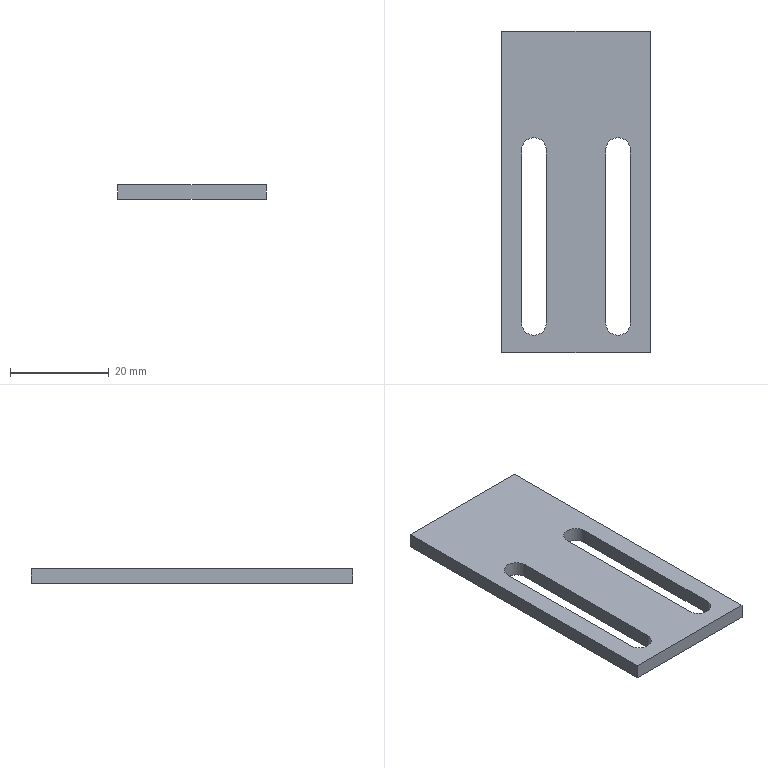Part | SolidWorks | features Extrusion 1, ICE 1, MirrorPattern 1 | 1 solid | 14 faces | box 30 x 65 x 3 mm | volume 4682 mm3 | plane 10 | cylinder 4 | commonest cylinder face diameters 5 x4
STEP:
#1=CARTESIAN_POINT('',(15.,-32.5,3.));
#2=VERTEX_POINT('',#1);
#3=CARTESIAN_POINT('',(15.,32.5,3.));
#4=VERTEX_POINT('',#3);
#5=CARTESIAN_POINT('',(15.,-32.5,3.));
#6=DIRECTION('',(0.,1.,0.));
#7=VECTOR('',#6,1000.);
#8=LINE('',#5,#7);
#9=EDGE_CURVE('',#2,#4,#8,.T.);
#10=ORIENTED_EDGE('',*,*,#9,.T.);
#11=CARTESIAN_POINT('',(-15.,32.5,3.));
#12=VERTEX_POINT('',#11);
#13=CARTESIAN_POINT('',(-15.,32.5,3.));
#14=DIRECTION('',(-1.,0.,0.));
#15=VECTOR('',#14,1000.);
#16=LINE('',#13,#15);
#17=EDGE_CURVE('',#4,#12,#16,.T.);
#18=ORIENTED_EDGE('',*,*,#17,.T.);
#19=CARTESIAN_POINT('',(-15.,-32.5,3.));
#20=VERTEX_POINT('',#19);
#21=CARTESIAN_POINT('',(-15.,-32.5,3.));
#22=DIRECTION('',(0.,-1.,0.));
#23=VECTOR('',#22,1000.);
#24=LINE('',#21,#23);
#25=EDGE_CURVE('',#12,#20,#24,.T.);
#26=ORIENTED_EDGE('',*,*,#25,.T.);
#27=CARTESIAN_POINT('',(-15.,-32.5,3.));
#28=DIRECTION('',(1.,0.,0.));
#29=VECTOR('',#28,1000.);
#30=LINE('',#27,#29);
#31=EDGE_CURVE('',#20,#2,#30,.T.);
#32=ORIENTED_EDGE('',*,*,#31,.T.);
#33=EDGE_LOOP('',(#10,#18,#26,#32));
#34=FACE_OUTER_BOUND('',#33,.T.);
#35=CARTESIAN_POINT('',(-6.,-26.5,3.));
#36=VERTEX_POINT('',#35);
#37=CARTESIAN_POINT('',(-6.,8.5,3.));
#38=VERTEX_POINT('',#37);
#39=CARTESIAN_POINT('',(-6.,-26.5,3.));
#40=DIRECTION('',(0.,1.,0.));
#41=VECTOR('',#40,1000.);
#42=LINE('',#39,#41);
#43=EDGE_CURVE('',#36,#38,#42,.T.);
#44=ORIENTED_EDGE('',*,*,#43,.F.);
#45=CARTESIAN_POINT('',(-11.,-26.5,3.));
#46=VERTEX_POINT('',#45);
#47=CARTESIAN_POINT('',(-8.5,-26.5,3.));
#48=DIRECTION('',(0.,0.,1.));
#49=DIRECTION('',(1.,0.,0.));
#50=AXIS2_PLACEMENT_3D('',#47,#48,#49);
#51=CIRCLE('',#50,2.5);
#52=EDGE_CURVE('',#46,#36,#51,.T.);
#53=ORIENTED_EDGE('',*,*,#52,.F.);
#54=CARTESIAN_POINT('',(-11.,8.5,3.));
#55=VERTEX_POINT('',#54);
#56=CARTESIAN_POINT('',(-11.,-26.5,3.));
#57=DIRECTION('',(0.,-1.,0.));
#58=VECTOR('',#57,1000.);
#59=LINE('',#56,#58);
#60=EDGE_CURVE('',#55,#46,#59,.T.);
#61=ORIENTED_EDGE('',*,*,#60,.F.);
#62=CARTESIAN_POINT('',(-8.5,8.5,3.));
#63=DIRECTION('',(0.,0.,1.));
#64=DIRECTION('',(1.,0.,0.));
#65=AXIS2_PLACEMENT_3D('',#62,#63,#64);
#66=CIRCLE('',#65,2.5);
#67=EDGE_CURVE('',#38,#55,#66,.T.);
#68=ORIENTED_EDGE('',*,*,#67,.F.);
#69=EDGE_LOOP('',(#44,#53,#61,#68));
#70=FACE_BOUND('',#69,.T.);
#71=CARTESIAN_POINT('',(11.,-26.5,3.));
#72=VERTEX_POINT('',#71);
#73=CARTESIAN_POINT('',(6.,-26.5,3.));
#74=VERTEX_POINT('',#73);
#75=CARTESIAN_POINT('',(8.5,-26.5,3.));
#76=DIRECTION('',(0.,0.,-1.));
#77=DIRECTION('',(-1.,0.,0.));
#78=AXIS2_PLACEMENT_3D('',#75,#76,#77);
#79=CIRCLE('',#78,2.5);
#80=EDGE_CURVE('',#72,#74,#79,.T.);
#81=ORIENTED_EDGE('',*,*,#80,.T.);
#82=CARTESIAN_POINT('',(6.,8.5,3.));
#83=VERTEX_POINT('',#82);
#84=CARTESIAN_POINT('',(6.,-26.5,3.));
#85=DIRECTION('',(0.,1.,0.));
#86=VECTOR('',#85,1000.);
#87=LINE('',#84,#86);
#88=EDGE_CURVE('',#74,#83,#87,.T.);
#89=ORIENTED_EDGE('',*,*,#88,.T.);
#90=CARTESIAN_POINT('',(11.,8.5,3.));
#91=VERTEX_POINT('',#90);
#92=CARTESIAN_POINT('',(8.5,8.5,3.));
#93=DIRECTION('',(0.,0.,-1.));
#94=DIRECTION('',(-1.,0.,0.));
#95=AXIS2_PLACEMENT_3D('',#92,#93,#94);
#96=CIRCLE('',#95,2.5);
#97=EDGE_CURVE('',#83,#91,#96,.T.);
#98=ORIENTED_EDGE('',*,*,#97,.T.);
#99=CARTESIAN_POINT('',(11.,-26.5,3.));
#100=DIRECTION('',(0.,-1.,0.));
#101=VECTOR('',#100,1000.);
#102=LINE('',#99,#101);
#103=EDGE_CURVE('',#91,#72,#102,.T.);
#104=ORIENTED_EDGE('',*,*,#103,.T.);
#105=EDGE_LOOP('',(#81,#89,#98,#104));
#106=FACE_BOUND('',#105,.T.);
#107=CARTESIAN_POINT('',(0.,0.,3.));
#108=DIRECTION('',(0.,0.,-1.));
#109=DIRECTION('',(-1.,0.,0.));
#110=AXIS2_PLACEMENT_3D('',#107,#108,#109);
#111=PLANE('',#110);
#112=ADVANCED_FACE('',(#34,#70,#106),#111,.F.);
#113=CARTESIAN_POINT('',(-11.,-26.5,0.));
#114=VERTEX_POINT('',#113);
#115=CARTESIAN_POINT('',(-6.,-26.5,0.));
#116=VERTEX_POINT('',#115);
#117=CARTESIAN_POINT('',(-8.5,-26.5,0.));
#118=DIRECTION('',(0.,0.,1.));
#119=DIRECTION('',(-1.,0.,0.));
#120=AXIS2_PLACEMENT_3D('',#117,#118,#119);
#121=CIRCLE('',#120,2.5);
#122=EDGE_CURVE('',#114,#116,#121,.T.);
#123=ORIENTED_EDGE('',*,*,#122,.T.);
#124=CARTESIAN_POINT('',(-6.,8.5,0.));
#125=VERTEX_POINT('',#124);
#126=CARTESIAN_POINT('',(-6.,-26.5,0.));
#127=DIRECTION('',(0.,1.,0.));
#128=VECTOR('',#127,1000.);
#129=LINE('',#126,#128);
#130=EDGE_CURVE('',#116,#125,#129,.T.);
#131=ORIENTED_EDGE('',*,*,#130,.T.);
#132=CARTESIAN_POINT('',(-11.,8.5,0.));
#133=VERTEX_POINT('',#132);
#134=CARTESIAN_POINT('',(-8.5,8.5,0.));
#135=DIRECTION('',(0.,0.,1.));
#136=DIRECTION('',(-1.,0.,0.));
#137=AXIS2_PLACEMENT_3D('',#134,#135,#136);
#138=CIRCLE('',#137,2.5);
#139=EDGE_CURVE('',#125,#133,#138,.T.);
#140=ORIENTED_EDGE('',*,*,#139,.T.);
#141=CARTESIAN_POINT('',(-11.,-26.5,0.));
#142=DIRECTION('',(0.,-1.,0.));
#143=VECTOR('',#142,1000.);
#144=LINE('',#141,#143);
#145=EDGE_CURVE('',#133,#114,#144,.T.);
#146=ORIENTED_EDGE('',*,*,#145,.T.);
#147=EDGE_LOOP('',(#123,#131,#140,#146));
#148=FACE_BOUND('',#147,.T.);
#149=CARTESIAN_POINT('',(15.,-32.5,0.));
#150=VERTEX_POINT('',#149);
#151=CARTESIAN_POINT('',(15.,32.5,0.));
#152=VERTEX_POINT('',#151);
#153=CARTESIAN_POINT('',(15.,-32.5,0.));
#154=DIRECTION('',(0.,1.,0.));
#155=VECTOR('',#154,1000.);
#156=LINE('',#153,#155);
#157=EDGE_CURVE('',#150,#152,#156,.T.);
#158=ORIENTED_EDGE('',*,*,#157,.F.);
#159=CARTESIAN_POINT('',(-15.,-32.5,0.));
#160=VERTEX_POINT('',#159);
#161=CARTESIAN_POINT('',(-15.,-32.5,0.));
#162=DIRECTION('',(1.,0.,0.));
#163=VECTOR('',#162,1000.);
#164=LINE('',#161,#163);
#165=EDGE_CURVE('',#160,#150,#164,.T.);
#166=ORIENTED_EDGE('',*,*,#165,.F.);
#167=CARTESIAN_POINT('',(-15.,32.5,0.));
#168=VERTEX_POINT('',#167);
#169=CARTESIAN_POINT('',(-15.,-32.5,0.));
#170=DIRECTION('',(0.,-1.,0.));
#171=VECTOR('',#170,1000.);
#172=LINE('',#169,#171);
#173=EDGE_CURVE('',#168,#160,#172,.T.);
#174=ORIENTED_EDGE('',*,*,#173,.F.);
#175=CARTESIAN_POINT('',(-15.,32.5,0.));
#176=DIRECTION('',(-1.,0.,0.));
#177=VECTOR('',#176,1000.);
#178=LINE('',#175,#177);
#179=EDGE_CURVE('',#152,#168,#178,.T.);
#180=ORIENTED_EDGE('',*,*,#179,.F.);
#181=EDGE_LOOP('',(#158,#166,#174,#180));
#182=FACE_OUTER_BOUND('',#181,.T.);
#183=CARTESIAN_POINT('',(6.,-26.5,0.));
#184=VERTEX_POINT('',#183);
#185=CARTESIAN_POINT('',(6.,8.5,0.));
#186=VERTEX_POINT('',#185);
#187=CARTESIAN_POINT('',(6.,-26.5,0.));
#188=DIRECTION('',(0.,1.,0.));
#189=VECTOR('',#188,1000.);
#190=LINE('',#187,#189);
#191=EDGE_CURVE('',#184,#186,#190,.T.);
#192=ORIENTED_EDGE('',*,*,#191,.F.);
#193=CARTESIAN_POINT('',(11.,-26.5,0.));
#194=VERTEX_POINT('',#193);
#195=CARTESIAN_POINT('',(8.5,-26.5,0.));
#196=DIRECTION('',(0.,0.,-1.));
#197=DIRECTION('',(-1.,0.,0.));
#198=AXIS2_PLACEMENT_3D('',#195,#196,#197);
#199=CIRCLE('',#198,2.5);
#200=EDGE_CURVE('',#194,#184,#199,.T.);
#201=ORIENTED_EDGE('',*,*,#200,.F.);
#202=CARTESIAN_POINT('',(11.,8.5,0.));
#203=VERTEX_POINT('',#202);
#204=CARTESIAN_POINT('',(11.,-26.5,0.));
#205=DIRECTION('',(0.,-1.,0.));
#206=VECTOR('',#205,1000.);
#207=LINE('',#204,#206);
#208=EDGE_CURVE('',#203,#194,#207,.T.);
#209=ORIENTED_EDGE('',*,*,#208,.F.);
#210=CARTESIAN_POINT('',(8.5,8.5,0.));
#211=DIRECTION('',(0.,0.,-1.));
#212=DIRECTION('',(-1.,0.,0.));
#213=AXIS2_PLACEMENT_3D('',#210,#211,#212);
#214=CIRCLE('',#213,2.5);
#215=EDGE_CURVE('',#186,#203,#214,.T.);
#216=ORIENTED_EDGE('',*,*,#215,.F.);
#217=EDGE_LOOP('',(#192,#201,#209,#216));
#218=FACE_BOUND('',#217,.T.);
#219=CARTESIAN_POINT('',(0.,0.,0.));
#220=DIRECTION('',(0.,0.,-1.));
#221=DIRECTION('',(-1.,0.,0.));
#222=AXIS2_PLACEMENT_3D('',#219,#220,#221);
#223=PLANE('',#222);
#224=ADVANCED_FACE('',(#148,#182,#218),#223,.T.);
#225=ORIENTED_EDGE('',*,*,#157,.T.);
#226=CARTESIAN_POINT('',(15.,32.5,3.));
#227=DIRECTION('',(0.,0.,-1.));
#228=VECTOR('',#227,1000.);
#229=LINE('',#226,#228);
#230=EDGE_CURVE('',#4,#152,#229,.T.);
#231=ORIENTED_EDGE('',*,*,#230,.F.);
#232=ORIENTED_EDGE('',*,*,#9,.F.);
#233=CARTESIAN_POINT('',(15.,-32.5,3.));
#234=DIRECTION('',(0.,0.,-1.));
#235=VECTOR('',#234,1000.);
#236=LINE('',#233,#235);
#237=EDGE_CURVE('',#2,#150,#236,.T.);
#238=ORIENTED_EDGE('',*,*,#237,.T.);
#239=EDGE_LOOP('',(#225,#231,#232,#238));
#240=FACE_OUTER_BOUND('',#239,.T.);
#241=CARTESIAN_POINT('',(15.,-32.5,3.));
#242=DIRECTION('',(-1.,0.,0.));
#243=DIRECTION('',(0.,0.,1.));
#244=AXIS2_PLACEMENT_3D('',#241,#242,#243);
#245=PLANE('',#244);
#246=ADVANCED_FACE('',(#240),#245,.F.);
#247=ORIENTED_EDGE('',*,*,#179,.T.);
#248=CARTESIAN_POINT('',(-15.,32.5,3.));
#249=DIRECTION('',(0.,0.,-1.));
#250=VECTOR('',#249,1000.);
#251=LINE('',#248,#250);
#252=EDGE_CURVE('',#12,#168,#251,.T.);
#253=ORIENTED_EDGE('',*,*,#252,.F.);
#254=ORIENTED_EDGE('',*,*,#17,.F.);
#255=ORIENTED_EDGE('',*,*,#230,.T.);
#256=EDGE_LOOP('',(#247,#253,#254,#255));
#257=FACE_OUTER_BOUND('',#256,.T.);
#258=CARTESIAN_POINT('',(-15.,32.5,3.));
#259=DIRECTION('',(0.,-1.,0.));
#260=DIRECTION('',(0.,0.,-1.));
#261=AXIS2_PLACEMENT_3D('',#258,#259,#260);
#262=PLANE('',#261);
#263=ADVANCED_FACE('',(#257),#262,.F.);
#264=ORIENTED_EDGE('',*,*,#173,.T.);
#265=CARTESIAN_POINT('',(-15.,-32.5,3.));
#266=DIRECTION('',(0.,0.,-1.));
#267=VECTOR('',#266,1000.);
#268=LINE('',#265,#267);
#269=EDGE_CURVE('',#20,#160,#268,.T.);
#270=ORIENTED_EDGE('',*,*,#269,.F.);
#271=ORIENTED_EDGE('',*,*,#25,.F.);
#272=ORIENTED_EDGE('',*,*,#252,.T.);
#273=EDGE_LOOP('',(#264,#270,#271,#272));
#274=FACE_OUTER_BOUND('',#273,.T.);
#275=CARTESIAN_POINT('',(-15.,-32.5,3.));
#276=DIRECTION('',(1.,0.,0.));
#277=DIRECTION('',(0.,0.,-1.));
#278=AXIS2_PLACEMENT_3D('',#275,#276,#277);
#279=PLANE('',#278);
#280=ADVANCED_FACE('',(#274),#279,.F.);
#281=ORIENTED_EDGE('',*,*,#165,.T.);
#282=ORIENTED_EDGE('',*,*,#237,.F.);
#283=ORIENTED_EDGE('',*,*,#31,.F.);
#284=ORIENTED_EDGE('',*,*,#269,.T.);
#285=EDGE_LOOP('',(#281,#282,#283,#284));
#286=FACE_OUTER_BOUND('',#285,.T.);
#287=CARTESIAN_POINT('',(-15.,-32.5,3.));
#288=DIRECTION('',(0.,1.,0.));
#289=DIRECTION('',(0.,0.,1.));
#290=AXIS2_PLACEMENT_3D('',#287,#288,#289);
#291=PLANE('',#290);
#292=ADVANCED_FACE('',(#286),#291,.F.);
#293=CARTESIAN_POINT('',(-11.,-26.5,-0.001));
#294=DIRECTION('',(0.,0.,1.));
#295=VECTOR('',#294,1000.);
#296=LINE('',#293,#295);
#297=EDGE_CURVE('',#114,#46,#296,.T.);
#298=ORIENTED_EDGE('',*,*,#297,.T.);
#299=ORIENTED_EDGE('',*,*,#52,.T.);
#300=CARTESIAN_POINT('',(-6.,-26.5,-0.001));
#301=DIRECTION('',(0.,0.,1.));
#302=VECTOR('',#301,1000.);
#303=LINE('',#300,#302);
#304=EDGE_CURVE('',#116,#36,#303,.T.);
#305=ORIENTED_EDGE('',*,*,#304,.F.);
#306=ORIENTED_EDGE('',*,*,#122,.F.);
#307=EDGE_LOOP('',(#298,#299,#305,#306));
#308=FACE_OUTER_BOUND('',#307,.T.);
#309=CARTESIAN_POINT('',(-8.5,-26.5,-0.001));
#310=DIRECTION('',(0.,0.,1.));
#311=DIRECTION('',(1.,0.,0.));
#312=AXIS2_PLACEMENT_3D('',#309,#310,#311);
#313=CYLINDRICAL_SURFACE('',#312,2.5);
#314=ADVANCED_FACE('',(#308),#313,.F.);
#315=CARTESIAN_POINT('',(-11.,8.5,-0.001));
#316=DIRECTION('',(0.,0.,1.));
#317=VECTOR('',#316,1000.);
#318=LINE('',#315,#317);
#319=EDGE_CURVE('',#133,#55,#318,.T.);
#320=ORIENTED_EDGE('',*,*,#319,.T.);
#321=ORIENTED_EDGE('',*,*,#60,.T.);
#322=ORIENTED_EDGE('',*,*,#297,.F.);
#323=ORIENTED_EDGE('',*,*,#145,.F.);
#324=EDGE_LOOP('',(#320,#321,#322,#323));
#325=FACE_OUTER_BOUND('',#324,.T.);
#326=CARTESIAN_POINT('',(-11.,-26.5,-0.001));
#327=DIRECTION('',(-1.,0.,0.));
#328=DIRECTION('',(0.,-1.,0.));
#329=AXIS2_PLACEMENT_3D('',#326,#327,#328);
#330=PLANE('',#329);
#331=ADVANCED_FACE('',(#325),#330,.F.);
#332=CARTESIAN_POINT('',(-6.,8.5,-0.001));
#333=DIRECTION('',(0.,0.,1.));
#334=VECTOR('',#333,1000.);
#335=LINE('',#332,#334);
#336=EDGE_CURVE('',#125,#38,#335,.T.);
#337=ORIENTED_EDGE('',*,*,#336,.T.);
#338=ORIENTED_EDGE('',*,*,#67,.T.);
#339=ORIENTED_EDGE('',*,*,#319,.F.);
#340=ORIENTED_EDGE('',*,*,#139,.F.);
#341=EDGE_LOOP('',(#337,#338,#339,#340));
#342=FACE_OUTER_BOUND('',#341,.T.);
#343=CARTESIAN_POINT('',(-8.5,8.5,-0.001));
#344=DIRECTION('',(0.,0.,1.));
#345=DIRECTION('',(1.,0.,0.));
#346=AXIS2_PLACEMENT_3D('',#343,#344,#345);
#347=CYLINDRICAL_SURFACE('',#346,2.5);
#348=ADVANCED_FACE('',(#342),#347,.F.);
#349=ORIENTED_EDGE('',*,*,#304,.T.);
#350=ORIENTED_EDGE('',*,*,#43,.T.);
#351=ORIENTED_EDGE('',*,*,#336,.F.);
#352=ORIENTED_EDGE('',*,*,#130,.F.);
#353=EDGE_LOOP('',(#349,#350,#351,#352));
#354=FACE_OUTER_BOUND('',#353,.T.);
#355=CARTESIAN_POINT('',(-6.,-26.5,-0.001));
#356=DIRECTION('',(1.,0.,0.));
#357=DIRECTION('',(0.,1.,0.));
#358=AXIS2_PLACEMENT_3D('',#355,#356,#357);
#359=PLANE('',#358);
#360=ADVANCED_FACE('',(#354),#359,.F.);
#361=ORIENTED_EDGE('',*,*,#200,.T.);
#362=CARTESIAN_POINT('',(6.,-26.5,-0.001));
#363=DIRECTION('',(0.,0.,1.));
#364=VECTOR('',#363,1000.);
#365=LINE('',#362,#364);
#366=EDGE_CURVE('',#184,#74,#365,.T.);
#367=ORIENTED_EDGE('',*,*,#366,.T.);
#368=ORIENTED_EDGE('',*,*,#80,.F.);
#369=CARTESIAN_POINT('',(11.,-26.5,-0.001));
#370=DIRECTION('',(0.,0.,1.));
#371=VECTOR('',#370,1000.);
#372=LINE('',#369,#371);
#373=EDGE_CURVE('',#194,#72,#372,.T.);
#374=ORIENTED_EDGE('',*,*,#373,.F.);
#375=EDGE_LOOP('',(#361,#367,#368,#374));
#376=FACE_OUTER_BOUND('',#375,.T.);
#377=CARTESIAN_POINT('',(8.5,-26.5,-0.001));
#378=DIRECTION('',(0.,0.,1.));
#379=DIRECTION('',(1.,0.,0.));
#380=AXIS2_PLACEMENT_3D('',#377,#378,#379);
#381=CYLINDRICAL_SURFACE('',#380,2.5);
#382=ADVANCED_FACE('',(#376),#381,.F.);
#383=ORIENTED_EDGE('',*,*,#191,.T.);
#384=CARTESIAN_POINT('',(6.,8.5,-0.001));
#385=DIRECTION('',(0.,0.,1.));
#386=VECTOR('',#385,1000.);
#387=LINE('',#384,#386);
#388=EDGE_CURVE('',#186,#83,#387,.T.);
#389=ORIENTED_EDGE('',*,*,#388,.T.);
#390=ORIENTED_EDGE('',*,*,#88,.F.);
#391=ORIENTED_EDGE('',*,*,#366,.F.);
#392=EDGE_LOOP('',(#383,#389,#390,#391));
#393=FACE_OUTER_BOUND('',#392,.T.);
#394=CARTESIAN_POINT('',(6.,-26.5,-0.001));
#395=DIRECTION('',(1.,0.,0.));
#396=DIRECTION('',(0.,1.,0.));
#397=AXIS2_PLACEMENT_3D('',#394,#395,#396);
#398=PLANE('',#397);
#399=ADVANCED_FACE('',(#393),#398,.T.);
#400=ORIENTED_EDGE('',*,*,#215,.T.);
#401=CARTESIAN_POINT('',(11.,8.5,-0.001));
#402=DIRECTION('',(0.,0.,1.));
#403=VECTOR('',#402,1000.);
#404=LINE('',#401,#403);
#405=EDGE_CURVE('',#203,#91,#404,.T.);
#406=ORIENTED_EDGE('',*,*,#405,.T.);
#407=ORIENTED_EDGE('',*,*,#97,.F.);
#408=ORIENTED_EDGE('',*,*,#388,.F.);
#409=EDGE_LOOP('',(#400,#406,#407,#408));
#410=FACE_OUTER_BOUND('',#409,.T.);
#411=CARTESIAN_POINT('',(8.5,8.5,-0.001));
#412=DIRECTION('',(0.,0.,1.));
#413=DIRECTION('',(1.,0.,0.));
#414=AXIS2_PLACEMENT_3D('',#411,#412,#413);
#415=CYLINDRICAL_SURFACE('',#414,2.5);
#416=ADVANCED_FACE('',(#410),#415,.F.);
#417=ORIENTED_EDGE('',*,*,#208,.T.);
#418=ORIENTED_EDGE('',*,*,#373,.T.);
#419=ORIENTED_EDGE('',*,*,#103,.F.);
#420=ORIENTED_EDGE('',*,*,#405,.F.);
#421=EDGE_LOOP('',(#417,#418,#419,#420));
#422=FACE_OUTER_BOUND('',#421,.T.);
#423=CARTESIAN_POINT('',(11.,-26.5,-0.001));
#424=DIRECTION('',(-1.,0.,0.));
#425=DIRECTION('',(0.,-1.,0.));
#426=AXIS2_PLACEMENT_3D('',#423,#424,#425);
#427=PLANE('',#426);
#428=ADVANCED_FACE('',(#422),#427,.T.);
#429=CLOSED_SHELL('',(#112,#224,#246,#263,#280,#292,#314,#331,#348,#360,#382,#399,#416,#428));
#430=MANIFOLD_SOLID_BREP('',#429);
#431=CARTESIAN_POINT('',(0.,0.,0.));
#432=DIRECTION('',(0.,0.,1.));
#433=DIRECTION('',(1.,0.,0.));
#434=AXIS2_PLACEMENT_3D('',#431,#432,#433);
#435=(LENGTH_UNIT()NAMED_UNIT(*)SI_UNIT(.MILLI.,.METRE.));
#436=UNCERTAINTY_MEASURE_WITH_UNIT(LENGTH_MEASURE(0.00001),#435,'','');
#437=(NAMED_UNIT(*)PLANE_ANGLE_UNIT()SI_UNIT($,.RADIAN.));
#438=(NAMED_UNIT(*)SI_UNIT($,.STERADIAN.)SOLID_ANGLE_UNIT());
#439=(GEOMETRIC_REPRESENTATION_CONTEXT(3)GLOBAL_UNCERTAINTY_ASSIGNED_CONTEXT((#436))GLOBAL_UNIT_ASSIGNED_CONTEXT((#435,#437,#438))REPRESENTATION_CONTEXT('',''));
#440=ADVANCED_BREP_SHAPE_REPRESENTATION('',(#430,#434),#439);